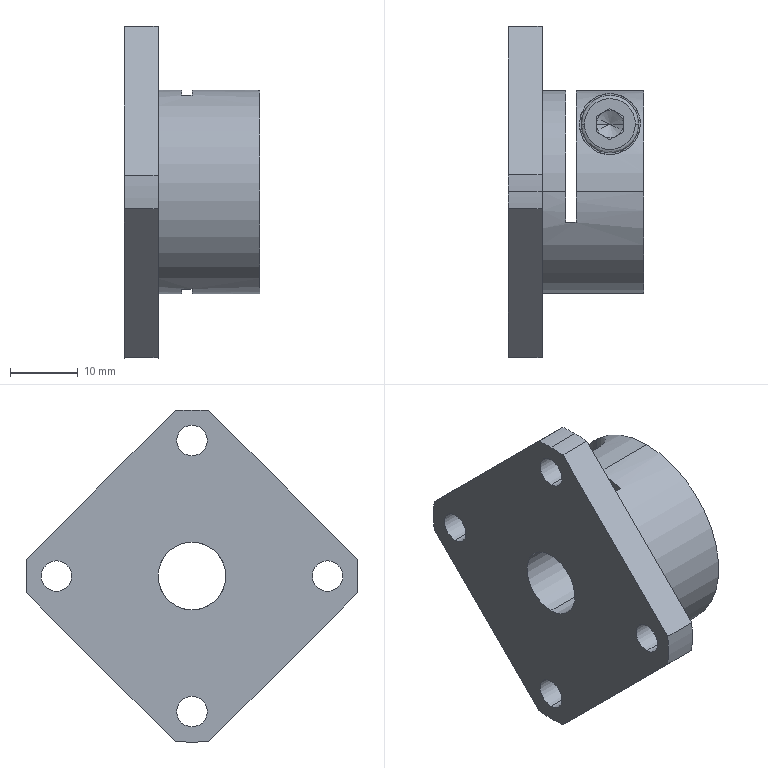Part | STEP file | Guide shaft support STHWS10 | 2 solids | 76 faces | box 20 x 49 x 49 mm | volume 14722 mm3 | plane 34 | cylinder 31 | cone 9 | spline 2 | commonest cylinder face diameters 4.5 x8 49 x5 10 x4 30 x4 4.134 x2 5 x2